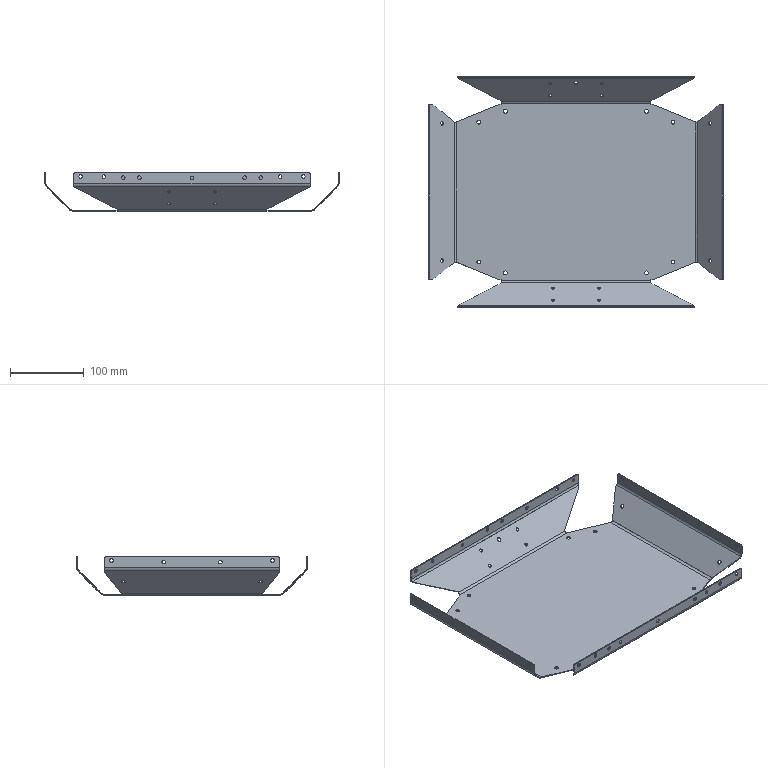Part | SolidWorks | features BaseBody 1 | 1 solid | 178 faces | box 400.001 x 314.942 x 51.999 mm | volume 169253 mm3 | cylinder 124 | plane 54 | commonest cylinder face diameters 4.9 x42 5.2 x34 4 x24 10 x12 12.4 x8 20 x4